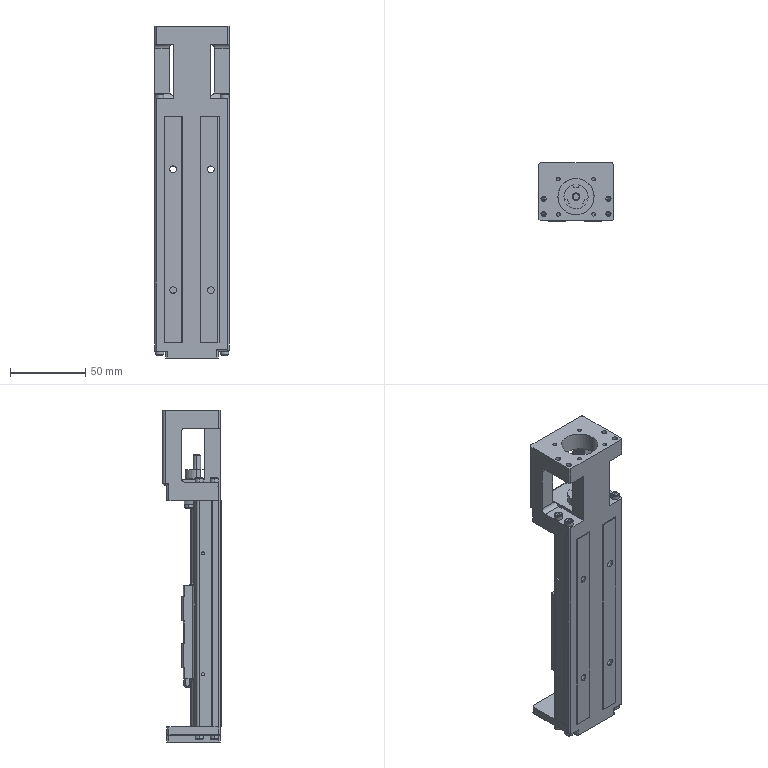Part | NX | features BREP 4 | 1 solid | 483 faces | box 50 x 38.5 x 220 mm | volume 169313 mm3 | plane 239 | cylinder 171 | cone 47 | torus 18 | spline 6 | sphere 2 | commonest cylinder face diameters 5.5 x32 2.5 x19 3 x16 6 x16 1 x12 2.15 x12